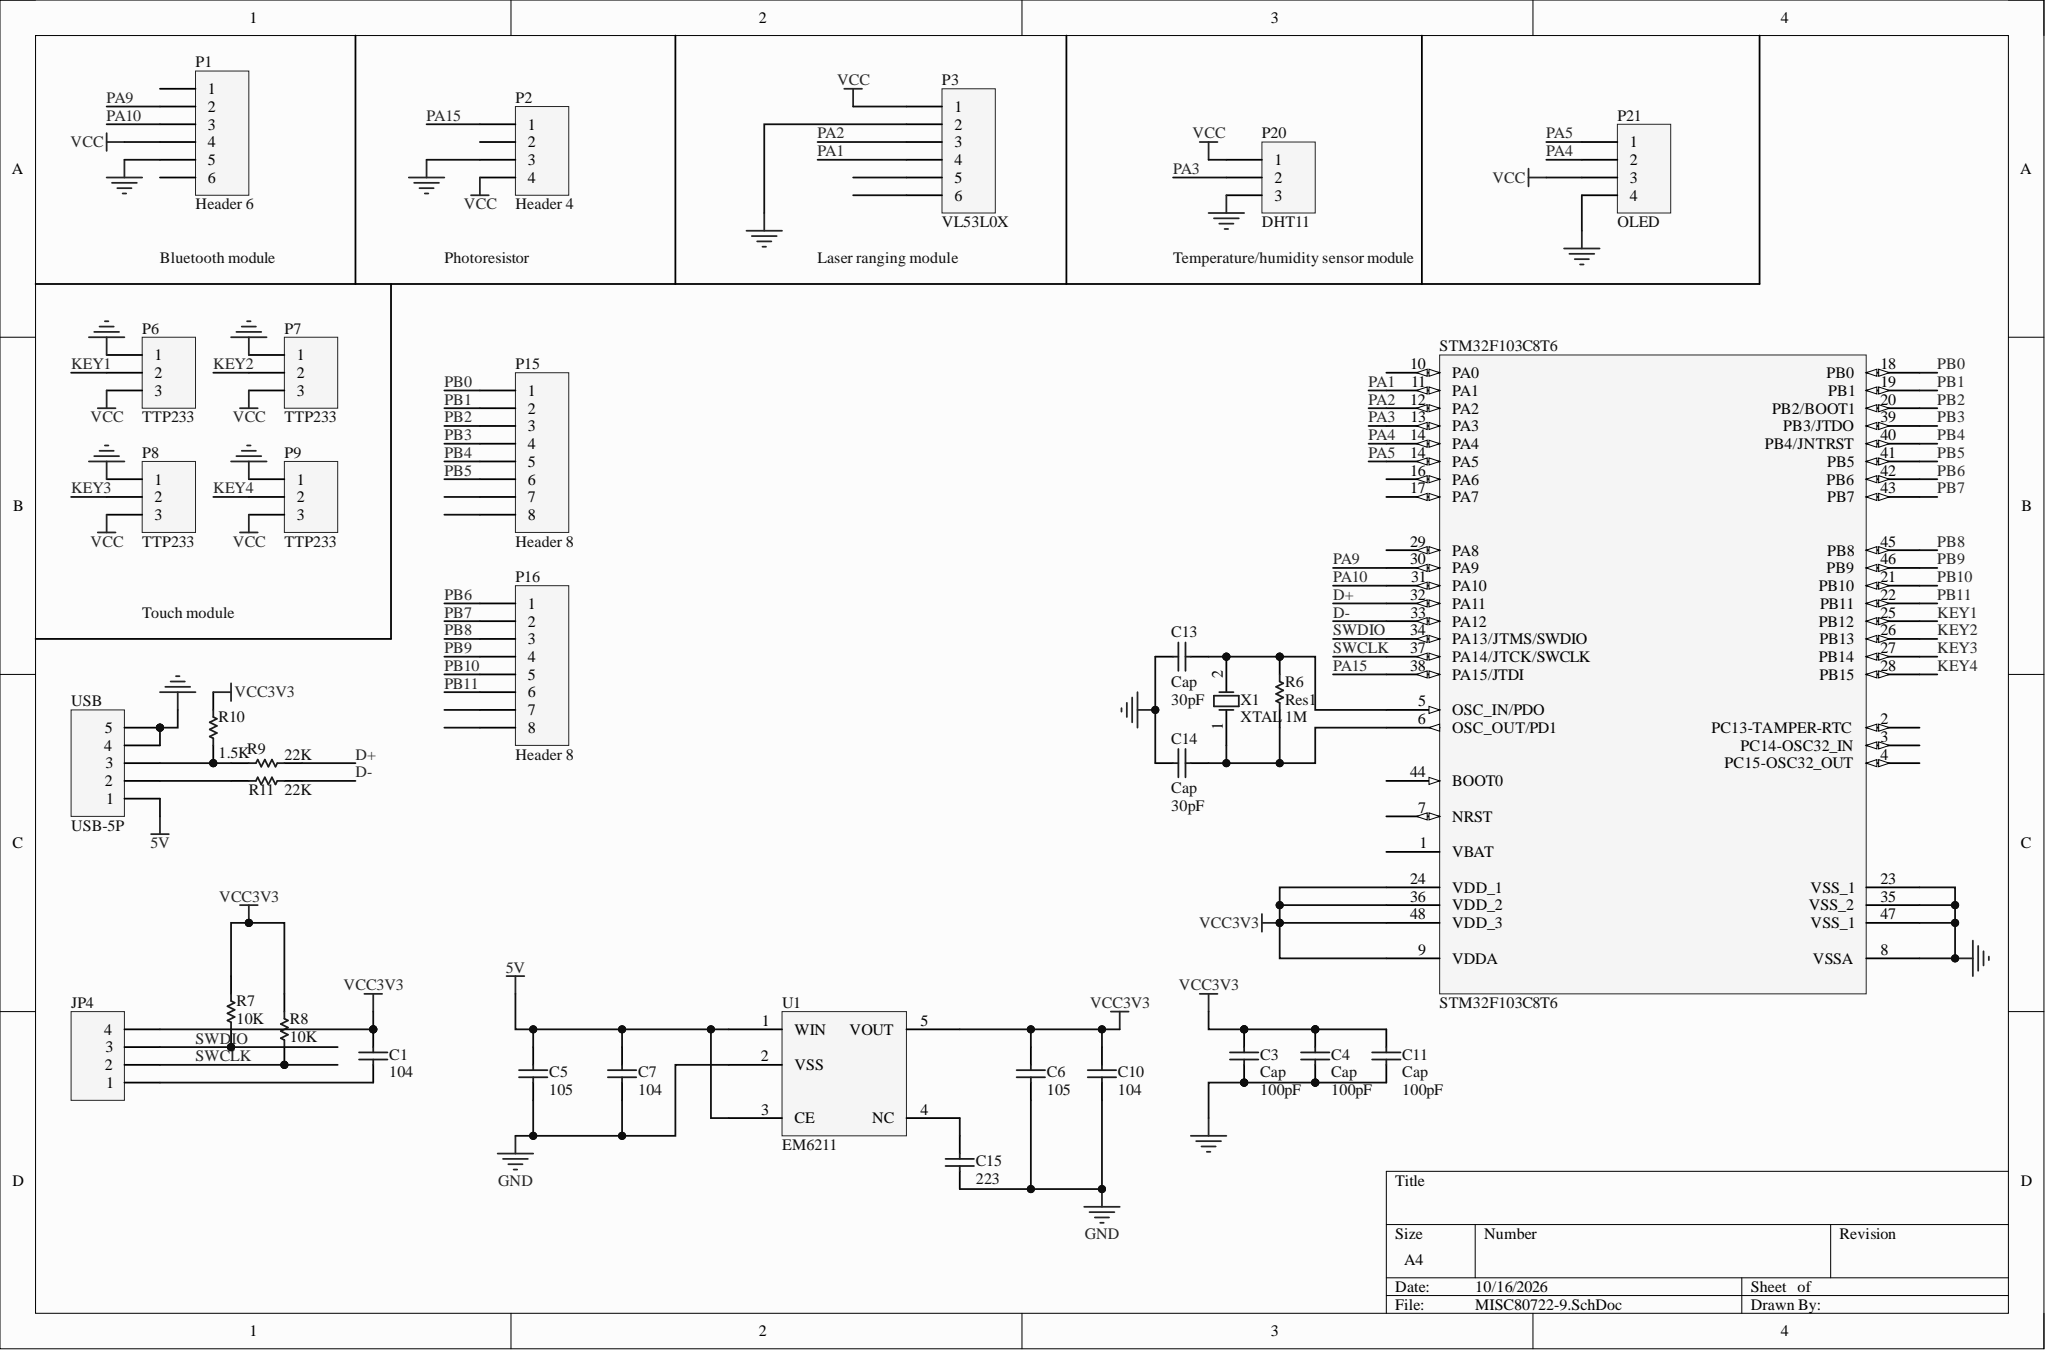Circuit board | Altium Designer | 33 parts | 38 nets
Bill of materials:
Comment,Description,Designator,Footprint,LibRef,Quantity
"104","Capacitor","C1, C7, C10","RAD-0.3","Cap","3"
"Cap","Capacitor","C3, C4, C11, C13, C14","RAD-0.3","Cap","5"
"105","Capacitor","C5, C6","RAD-0.3","Cap","2"
"223","Capacitor","C15","RAD-0.3","Cap","1"
"Header 4","Header, 4-Pin","JP4, P2","HDR1X4","Header 4","2"
"Header 6","Header, 6-Pin","P1","HDR1X6","Header 6","1"
"VL53L0X","Header, 6-Pin","P3","HDR1X6","Header 6","1"
"TTP233","Header, 3-Pin","P6, P7, P8, P9","HDR1X3","Header 3","4"
"Header 8","Header, 8-Pin","P15, P16","HDR1X8","Header 8","2"
"DHT11","Header, 3-Pin","P20","HDR1X3","Header 3","1"
"OLED","Header, 4-Pin","P21","HDR1X4","Header 4","1"
"Res1","Resistor","R6, R7, R8, R9, R10, R11","AXIAL-0.3","Res1","6"
"STM32F103C8T6","","STM32F103C8T6","PCBComponent_1","Component_1","1"
"EM6211","","U1","ME6211C28M5G","EM6211","1"
"USB-5P","Header, 5-Pin","USB","HDR1X5","Header 5","1"
"XTAL","Crystal Oscillator","X1","R38","XTAL","1"
Netlist (Protel format):
[
C1
RAD-0.3
104



]
[
C3
RAD-0.3
Cap



]
[
C4
RAD-0.3
Cap



]
[
C5
RAD-0.3
105



]
[
C6
RAD-0.3
105



]
[
C7
RAD-0.3
104



]
[
C10
RAD-0.3
104



]
[
C11
RAD-0.3
Cap



]
[
C13
RAD-0.3
Cap



]
[
C14
RAD-0.3
Cap



]
[
C15
RAD-0.3
223



]
[
JP4
HDR1X4
Header 4



]
[
P1
HDR1X6
Header 6



]
[
P2
HDR1X4
Header 4



]
[
P3
HDR1X6
VL53L0X



]
[
P6
HDR1X3
TTP233



]
[
P7
HDR1X3
TTP233



]
[
P8
HDR1X3
TTP233



]
[
P9
HDR1X3
TTP233



]
[
P15
HDR1X8
Header 8



]
[
P16
HDR1X8
Header 8



]
[
P20
HDR1X3
DHT11



]
[
P21
HDR1X4
OLED



]
[
R6
AXIAL-0.3
Res1



]
[
R7
AXIAL-0.3
Res1



]
[
R8
AXIAL-0.3
Res1



]
[
R9
AXIAL-0.3
Res1



]
[
R10
AXIAL-0.3
Res1



]
[
R11
AXIAL-0.3
Res1



]
[
STM32F103C8T6
PCBComponent_1
STM32F103C8T6



]
[
U1
ME6211C28M5G
EM6211



]
[
USB
HDR1X5
USB-5P



]
[
X1
R38
XTAL



]
(
VCC3V3
C1-2
C3-2
C4-2
C6-2
C10-2
C11-2
JP4-4
R7-1
R8-1
R10-2
STM32F103C8T6-9
STM32F103C8T6-24
STM32F103C8T6-36
STM32F103C8T6-48
U1-5
)
(
VCC
P1-4
P2-4
P3-1
P6-3
P7-3
P8-3
P9-3
P20-1
P21-3
)
(
SWDIO
JP4-3
R7-2
STM32F103C8T6-34
)
(
SWCLK
JP4-2
R8-2
STM32F103C8T6-37
)
(
PB11
P16-6
STM32F103C8T6-22
)
(
PB10
P16-5
STM32F103C8T6-21
)
(
PB9
P16-4
STM32F103C8T6-46
)
(
PB8
P16-3
STM32F103C8T6-45
)
(
PB7
P16-2
STM32F103C8T6-43
)
(
PB6
P16-1
STM32F103C8T6-42
)
(
PB5
P15-6
STM32F103C8T6-41
)
(
PB4
P15-5
STM32F103C8T6-40
)
(
PB3
P15-4
STM32F103C8T6-39
)
(
PB2
P15-3
STM32F103C8T6-20
)
(
PB1
P15-2
STM32F103C8T6-19
)
(
PB0
P15-1
STM32F103C8T6-18
)
(
PA15
P2-1
STM32F103C8T6-38
)
(
PA10
P1-3
STM32F103C8T6-31
)
(
PA9
P1-2
STM32F103C8T6-30
)
(
PA5
P21-1
STM32F103C8T6-14
)
(
PA4
P21-2
STM32F103C8T6-14
)
(
PA3
P20-2
STM32F103C8T6-13
)
(
PA2
P3-3
STM32F103C8T6-12
)
(
PA1
P3-4
STM32F103C8T6-11
)
(
NetR11_2
R11-2
USB-2
)
(
NetR9_2
R9-2
R10-1
USB-3
)
(
NetC15_2
C15-2
U1-4
)
(
NetC14_1
C14-1
R6-1
STM32F103C8T6-6
X1-1
)
(
NetC13_1
C13-1
R6-2
STM32F103C8T6-5
X1-2
)
(
NetC1_1
C1-1
JP4-1
)
(
KEY4
P9-2
STM32F103C8T6-28
)
(
KEY3
P8-2
STM32F103C8T6-27
)
(
KEY2
P7-2
STM32F103C8T6-26
)
(
KEY1
P6-2
STM32F103C8T6-25
)
(
GND
C3-1
C4-1
C5-1
C6-1
C7-1
C10-1
C11-1
C13-2
C14-2
C15-1
P1-5
P2-3
P3-2
P6-1
P7-1
P8-1
P9-1
P20-3
P21-4
STM32F103C8T6-8
STM32F103C8T6-23
STM32F103C8T6-35
STM32F103C8T6-47
U1-2
USB-4
USB-5
)
(
D-
R11-1
STM32F103C8T6-33
)
(
D+
R9-1
STM32F103C8T6-32
)
(
5V
C5-2
C7-2
U1-1
U1-3
USB-1
)